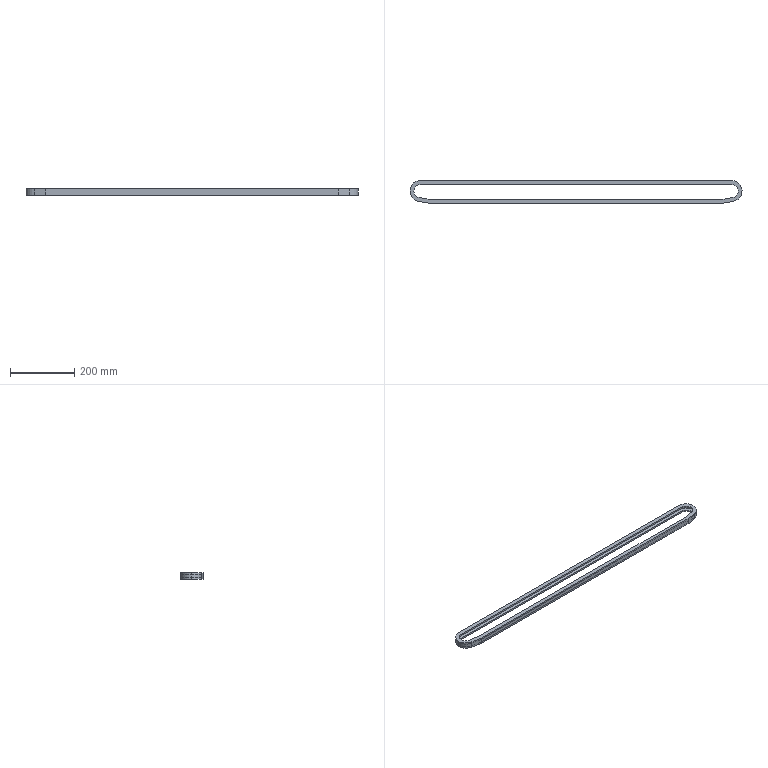Part | SolidWorks | features Extrusion 1, ICE 1 | 1 solid | 32 faces | box 1035 x 70.699 x 20 mm | volume 274324 mm3 | plane 20 | cylinder 12 | commonest cylinder face diameters 41 x6 63 x3 65 x3
STEP:
#1=CARTESIAN_POINT('',(516.5,0.,-5.));
#2=VERTEX_POINT('',#1);
#3=CARTESIAN_POINT('',(485.,31.5,-5.));
#4=VERTEX_POINT('',#3);
#5=CARTESIAN_POINT('',(485.,0.,-5.));
#6=DIRECTION('',(0.,0.,1.));
#7=DIRECTION('',(1.,0.,0.));
#8=AXIS2_PLACEMENT_3D('',#5,#6,#7);
#9=CIRCLE('',#8,31.5);
#10=EDGE_CURVE('',#2,#4,#9,.T.);
#11=ORIENTED_EDGE('',*,*,#10,.F.);
#12=CARTESIAN_POINT('',(516.5,0.,5.));
#13=VERTEX_POINT('',#12);
#14=CARTESIAN_POINT('',(516.5,0.,-5.));
#15=DIRECTION('',(0.,0.,1.));
#16=VECTOR('',#15,1000.);
#17=LINE('',#14,#16);
#18=EDGE_CURVE('',#2,#13,#17,.T.);
#19=ORIENTED_EDGE('',*,*,#18,.T.);
#20=CARTESIAN_POINT('',(485.,31.5,5.));
#21=VERTEX_POINT('',#20);
#22=CARTESIAN_POINT('',(485.,0.,5.));
#23=DIRECTION('',(0.,0.,1.));
#24=DIRECTION('',(1.,0.,0.));
#25=AXIS2_PLACEMENT_3D('',#22,#23,#24);
#26=CIRCLE('',#25,31.5);
#27=EDGE_CURVE('',#13,#21,#26,.T.);
#28=ORIENTED_EDGE('',*,*,#27,.T.);
#29=CARTESIAN_POINT('',(485.,31.5,-5.));
#30=DIRECTION('',(0.,0.,1.));
#31=VECTOR('',#30,1000.);
#32=LINE('',#29,#31);
#33=EDGE_CURVE('',#4,#21,#32,.T.);
#34=ORIENTED_EDGE('',*,*,#33,.F.);
#35=EDGE_LOOP('',(#11,#19,#28,#34));
#36=FACE_OUTER_BOUND('',#35,.T.);
#37=CARTESIAN_POINT('',(485.,0.,-5.));
#38=DIRECTION('',(0.,0.,1.));
#39=DIRECTION('',(1.,0.,0.));
#40=AXIS2_PLACEMENT_3D('',#37,#38,#39);
#41=CYLINDRICAL_SURFACE('',#40,31.5);
#42=ADVANCED_FACE('',(#36),#41,.F.);
#43=CARTESIAN_POINT('',(-485.,20.5,10.));
#44=VERTEX_POINT('',#43);
#45=CARTESIAN_POINT('',(-505.5,0.,10.));
#46=VERTEX_POINT('',#45);
#47=CARTESIAN_POINT('',(-485.,0.,10.));
#48=DIRECTION('',(0.,0.,1.));
#49=DIRECTION('',(1.,0.,0.));
#50=AXIS2_PLACEMENT_3D('',#47,#48,#49);
#51=CIRCLE('',#50,20.5);
#52=EDGE_CURVE('',#44,#46,#51,.T.);
#53=ORIENTED_EDGE('',*,*,#52,.T.);
#54=CARTESIAN_POINT('',(-505.5,0.,5.));
#55=VERTEX_POINT('',#54);
#56=CARTESIAN_POINT('',(-505.5,0.,10.));
#57=DIRECTION('',(0.,0.,-1.));
#58=VECTOR('',#57,1000.);
#59=LINE('',#56,#58);
#60=EDGE_CURVE('',#46,#55,#59,.T.);
#61=ORIENTED_EDGE('',*,*,#60,.T.);
#62=CARTESIAN_POINT('',(-485.,20.5,5.));
#63=VERTEX_POINT('',#62);
#64=CARTESIAN_POINT('',(-485.,0.,5.));
#65=DIRECTION('',(0.,0.,1.));
#66=DIRECTION('',(1.,0.,0.));
#67=AXIS2_PLACEMENT_3D('',#64,#65,#66);
#68=CIRCLE('',#67,20.5);
#69=EDGE_CURVE('',#63,#55,#68,.T.);
#70=ORIENTED_EDGE('',*,*,#69,.F.);
#71=CARTESIAN_POINT('',(-485.,20.5,10.));
#72=DIRECTION('',(0.,0.,-1.));
#73=VECTOR('',#72,1000.);
#74=LINE('',#71,#73);
#75=EDGE_CURVE('',#44,#63,#74,.T.);
#76=ORIENTED_EDGE('',*,*,#75,.F.);
#77=EDGE_LOOP('',(#53,#61,#70,#76));
#78=FACE_OUTER_BOUND('',#77,.T.);
#79=CARTESIAN_POINT('',(-485.,0.,10.));
#80=DIRECTION('',(0.,0.,-1.));
#81=DIRECTION('',(-1.,0.,0.));
#82=AXIS2_PLACEMENT_3D('',#79,#80,#81);
#83=CYLINDRICAL_SURFACE('',#82,20.5);
#84=ADVANCED_FACE('',(#78),#83,.F.);
#85=CARTESIAN_POINT('',(-517.5,0.,10.));
#86=VERTEX_POINT('',#85);
#87=CARTESIAN_POINT('',(-490.644,-32.006,10.));
#88=VERTEX_POINT('',#87);
#89=CARTESIAN_POINT('',(-485.,0.,10.));
#90=DIRECTION('',(0.,0.,1.));
#91=DIRECTION('',(1.,0.,0.));
#92=AXIS2_PLACEMENT_3D('',#89,#90,#91);
#93=CIRCLE('',#92,32.5);
#94=EDGE_CURVE('',#86,#88,#93,.T.);
#95=ORIENTED_EDGE('',*,*,#94,.F.);
#96=CARTESIAN_POINT('',(-517.5,0.,-10.));
#97=VERTEX_POINT('',#96);
#98=CARTESIAN_POINT('',(-517.5,0.,10.));
#99=DIRECTION('',(0.,0.,-1.));
#100=VECTOR('',#99,1000.);
#101=LINE('',#98,#100);
#102=EDGE_CURVE('',#86,#97,#101,.T.);
#103=ORIENTED_EDGE('',*,*,#102,.T.);
#104=CARTESIAN_POINT('',(-490.644,-32.006,-10.));
#105=VERTEX_POINT('',#104);
#106=CARTESIAN_POINT('',(-485.,0.,-10.));
#107=DIRECTION('',(0.,0.,1.));
#108=DIRECTION('',(1.,0.,0.));
#109=AXIS2_PLACEMENT_3D('',#106,#107,#108);
#110=CIRCLE('',#109,32.5);
#111=EDGE_CURVE('',#97,#105,#110,.T.);
#112=ORIENTED_EDGE('',*,*,#111,.T.);
#113=CARTESIAN_POINT('',(-490.644,-32.006,10.));
#114=DIRECTION('',(0.,0.,-1.));
#115=VECTOR('',#114,1000.);
#116=LINE('',#113,#115);
#117=EDGE_CURVE('',#88,#105,#116,.T.);
#118=ORIENTED_EDGE('',*,*,#117,.F.);
#119=EDGE_LOOP('',(#95,#103,#112,#118));
#120=FACE_OUTER_BOUND('',#119,.T.);
#121=CARTESIAN_POINT('',(-485.,0.,10.));
#122=DIRECTION('',(0.,0.,-1.));
#123=DIRECTION('',(-1.,0.,0.));
#124=AXIS2_PLACEMENT_3D('',#121,#122,#123);
#125=CYLINDRICAL_SURFACE('',#124,32.5);
#126=ADVANCED_FACE('',(#120),#125,.T.);
#127=CARTESIAN_POINT('',(-485.,20.5,-5.));
#128=VERTEX_POINT('',#127);
#129=CARTESIAN_POINT('',(-505.5,0.,-5.));
#130=VERTEX_POINT('',#129);
#131=CARTESIAN_POINT('',(-485.,0.,-5.));
#132=DIRECTION('',(0.,0.,1.));
#133=DIRECTION('',(1.,0.,0.));
#134=AXIS2_PLACEMENT_3D('',#131,#132,#133);
#135=CIRCLE('',#134,20.5);
#136=EDGE_CURVE('',#128,#130,#135,.T.);
#137=ORIENTED_EDGE('',*,*,#136,.T.);
#138=CARTESIAN_POINT('',(-505.5,0.,-10.));
#139=VERTEX_POINT('',#138);
#140=CARTESIAN_POINT('',(-505.5,0.,10.));
#141=DIRECTION('',(0.,0.,-1.));
#142=VECTOR('',#141,1000.);
#143=LINE('',#140,#142);
#144=EDGE_CURVE('',#130,#139,#143,.T.);
#145=ORIENTED_EDGE('',*,*,#144,.T.);
#146=CARTESIAN_POINT('',(-485.,20.5,-10.));
#147=VERTEX_POINT('',#146);
#148=CARTESIAN_POINT('',(-485.,0.,-10.));
#149=DIRECTION('',(0.,0.,1.));
#150=DIRECTION('',(1.,0.,0.));
#151=AXIS2_PLACEMENT_3D('',#148,#149,#150);
#152=CIRCLE('',#151,20.5);
#153=EDGE_CURVE('',#147,#139,#152,.T.);
#154=ORIENTED_EDGE('',*,*,#153,.F.);
#155=CARTESIAN_POINT('',(-485.,20.5,10.));
#156=DIRECTION('',(0.,0.,-1.));
#157=VECTOR('',#156,1000.);
#158=LINE('',#155,#157);
#159=EDGE_CURVE('',#128,#147,#158,.T.);
#160=ORIENTED_EDGE('',*,*,#159,.F.);
#161=EDGE_LOOP('',(#137,#145,#154,#160));
#162=FACE_OUTER_BOUND('',#161,.T.);
#163=CARTESIAN_POINT('',(-485.,0.,10.));
#164=DIRECTION('',(0.,0.,-1.));
#165=DIRECTION('',(-1.,0.,0.));
#166=AXIS2_PLACEMENT_3D('',#163,#164,#165);
#167=CYLINDRICAL_SURFACE('',#166,20.5);
#168=ADVANCED_FACE('',(#162),#167,.F.);
#169=ORIENTED_EDGE('',*,*,#144,.F.);
#170=CARTESIAN_POINT('',(-488.56,-20.189,-5.));
#171=VERTEX_POINT('',#170);
#172=CARTESIAN_POINT('',(-485.,0.,-5.));
#173=DIRECTION('',(0.,0.,1.));
#174=DIRECTION('',(1.,0.,0.));
#175=AXIS2_PLACEMENT_3D('',#172,#173,#174);
#176=CIRCLE('',#175,20.5);
#177=EDGE_CURVE('',#130,#171,#176,.T.);
#178=ORIENTED_EDGE('',*,*,#177,.T.);
#179=CARTESIAN_POINT('',(-488.56,-20.189,-10.));
#180=VERTEX_POINT('',#179);
#181=CARTESIAN_POINT('',(-488.56,-20.189,10.));
#182=DIRECTION('',(0.,0.,-1.));
#183=VECTOR('',#182,1000.);
#184=LINE('',#181,#183);
#185=EDGE_CURVE('',#171,#180,#184,.T.);
#186=ORIENTED_EDGE('',*,*,#185,.T.);
#187=CARTESIAN_POINT('',(-485.,0.,-10.));
#188=DIRECTION('',(0.,0.,1.));
#189=DIRECTION('',(1.,0.,0.));
#190=AXIS2_PLACEMENT_3D('',#187,#188,#189);
#191=CIRCLE('',#190,20.5);
#192=EDGE_CURVE('',#139,#180,#191,.T.);
#193=ORIENTED_EDGE('',*,*,#192,.F.);
#194=EDGE_LOOP('',(#169,#178,#186,#193));
#195=FACE_OUTER_BOUND('',#194,.T.);
#196=CARTESIAN_POINT('',(-485.,0.,10.));
#197=DIRECTION('',(0.,0.,-1.));
#198=DIRECTION('',(-1.,0.,0.));
#199=AXIS2_PLACEMENT_3D('',#196,#197,#198);
#200=CYLINDRICAL_SURFACE('',#199,20.5);
#201=ADVANCED_FACE('',(#195),#200,.F.);
#202=ORIENTED_EDGE('',*,*,#185,.F.);
#203=CARTESIAN_POINT('',(-454.475,-26.199,-5.));
#204=VERTEX_POINT('',#203);
#205=CARTESIAN_POINT('',(-454.475,-26.199,-5.));
#206=DIRECTION('',(0.9848,-0.1736,0.));
#207=VECTOR('',#206,1000.);
#208=LINE('',#205,#207);
#209=EDGE_CURVE('',#171,#204,#208,.T.);
#210=ORIENTED_EDGE('',*,*,#209,.T.);
#211=CARTESIAN_POINT('',(-454.475,-26.199,-10.));
#212=VERTEX_POINT('',#211);
#213=CARTESIAN_POINT('',(-454.475,-26.199,10.));
#214=DIRECTION('',(0.,0.,-1.));
#215=VECTOR('',#214,1000.);
#216=LINE('',#213,#215);
#217=EDGE_CURVE('',#204,#212,#216,.T.);
#218=ORIENTED_EDGE('',*,*,#217,.T.);
#219=CARTESIAN_POINT('',(-454.475,-26.199,-10.));
#220=DIRECTION('',(0.9848,-0.1736,0.));
#221=VECTOR('',#220,1000.);
#222=LINE('',#219,#221);
#223=EDGE_CURVE('',#180,#212,#222,.T.);
#224=ORIENTED_EDGE('',*,*,#223,.F.);
#225=EDGE_LOOP('',(#202,#210,#218,#224));
#226=FACE_OUTER_BOUND('',#225,.T.);
#227=CARTESIAN_POINT('',(-454.475,-26.199,10.));
#228=DIRECTION('',(0.1736,0.9848,0.));
#229=DIRECTION('',(-0.9848,0.1736,0.));
#230=AXIS2_PLACEMENT_3D('',#227,#228,#229);
#231=PLANE('',#230);
#232=ADVANCED_FACE('',(#226),#231,.T.);
#233=ORIENTED_EDGE('',*,*,#217,.F.);
#234=CARTESIAN_POINT('',(454.475,-26.199,-5.));
#235=VERTEX_POINT('',#234);
#236=CARTESIAN_POINT('',(-454.475,-26.199,-5.));
#237=DIRECTION('',(1.,0.,0.));
#238=VECTOR('',#237,1000.);
#239=LINE('',#236,#238);
#240=EDGE_CURVE('',#204,#235,#239,.T.);
#241=ORIENTED_EDGE('',*,*,#240,.T.);
#242=CARTESIAN_POINT('',(454.475,-26.199,-10.));
#243=VERTEX_POINT('',#242);
#244=CARTESIAN_POINT('',(454.475,-26.199,10.));
#245=DIRECTION('',(0.,0.,-1.));
#246=VECTOR('',#245,1000.);
#247=LINE('',#244,#246);
#248=EDGE_CURVE('',#235,#243,#247,.T.);
#249=ORIENTED_EDGE('',*,*,#248,.T.);
#250=CARTESIAN_POINT('',(-454.475,-26.199,-10.));
#251=DIRECTION('',(1.,0.,0.));
#252=VECTOR('',#251,1000.);
#253=LINE('',#250,#252);
#254=EDGE_CURVE('',#212,#243,#253,.T.);
#255=ORIENTED_EDGE('',*,*,#254,.F.);
#256=EDGE_LOOP('',(#233,#241,#249,#255));
#257=FACE_OUTER_BOUND('',#256,.T.);
#258=CARTESIAN_POINT('',(-454.475,-26.199,10.));
#259=DIRECTION('',(0.,1.,0.));
#260=DIRECTION('',(0.,0.,1.));
#261=AXIS2_PLACEMENT_3D('',#258,#259,#260);
#262=PLANE('',#261);
#263=ADVANCED_FACE('',(#257),#262,.T.);
#264=ORIENTED_EDGE('',*,*,#248,.F.);
#265=CARTESIAN_POINT('',(488.56,-20.189,-5.));
#266=VERTEX_POINT('',#265);
#267=CARTESIAN_POINT('',(454.475,-26.199,-5.));
#268=DIRECTION('',(0.9848,0.1736,0.));
#269=VECTOR('',#268,1000.);
#270=LINE('',#267,#269);
#271=EDGE_CURVE('',#235,#266,#270,.T.);
#272=ORIENTED_EDGE('',*,*,#271,.T.);
#273=CARTESIAN_POINT('',(488.56,-20.189,-10.));
#274=VERTEX_POINT('',#273);
#275=CARTESIAN_POINT('',(488.56,-20.189,10.));
#276=DIRECTION('',(0.,0.,-1.));
#277=VECTOR('',#276,1000.);
#278=LINE('',#275,#277);
#279=EDGE_CURVE('',#266,#274,#278,.T.);
#280=ORIENTED_EDGE('',*,*,#279,.T.);
#281=CARTESIAN_POINT('',(454.475,-26.199,-10.));
#282=DIRECTION('',(0.9848,0.1736,0.));
#283=VECTOR('',#282,1000.);
#284=LINE('',#281,#283);
#285=EDGE_CURVE('',#243,#274,#284,.T.);
#286=ORIENTED_EDGE('',*,*,#285,.F.);
#287=EDGE_LOOP('',(#264,#272,#280,#286));
#288=FACE_OUTER_BOUND('',#287,.T.);
#289=CARTESIAN_POINT('',(454.475,-26.199,10.));
#290=DIRECTION('',(-0.1736,0.9848,0.));
#291=DIRECTION('',(-0.9848,-0.1736,0.));
#292=AXIS2_PLACEMENT_3D('',#289,#290,#291);
#293=PLANE('',#292);
#294=ADVANCED_FACE('',(#288),#293,.T.);
#295=ORIENTED_EDGE('',*,*,#279,.F.);
#296=CARTESIAN_POINT('',(485.,20.5,-5.));
#297=VERTEX_POINT('',#296);
#298=CARTESIAN_POINT('',(485.,0.,-5.));
#299=DIRECTION('',(0.,0.,1.));
#300=DIRECTION('',(1.,0.,0.));
#301=AXIS2_PLACEMENT_3D('',#298,#299,#300);
#302=CIRCLE('',#301,20.5);
#303=EDGE_CURVE('',#266,#297,#302,.T.);
#304=ORIENTED_EDGE('',*,*,#303,.T.);
#305=CARTESIAN_POINT('',(485.,20.5,-10.));
#306=VERTEX_POINT('',#305);
#307=CARTESIAN_POINT('',(485.,20.5,10.));
#308=DIRECTION('',(0.,0.,-1.));
#309=VECTOR('',#308,1000.);
#310=LINE('',#307,#309);
#311=EDGE_CURVE('',#297,#306,#310,.T.);
#312=ORIENTED_EDGE('',*,*,#311,.T.);
#313=CARTESIAN_POINT('',(485.,0.,-10.));
#314=DIRECTION('',(0.,0.,1.));
#315=DIRECTION('',(-1.,0.,0.));
#316=AXIS2_PLACEMENT_3D('',#313,#314,#315);
#317=CIRCLE('',#316,20.5);
#318=EDGE_CURVE('',#274,#306,#317,.T.);
#319=ORIENTED_EDGE('',*,*,#318,.F.);
#320=EDGE_LOOP('',(#295,#304,#312,#319));
#321=FACE_OUTER_BOUND('',#320,.T.);
#322=CARTESIAN_POINT('',(485.,0.,10.));
#323=DIRECTION('',(0.,0.,-1.));
#324=DIRECTION('',(-1.,0.,0.));
#325=AXIS2_PLACEMENT_3D('',#322,#323,#324);
#326=CYLINDRICAL_SURFACE('',#325,20.5);
#327=ADVANCED_FACE('',(#321),#326,.F.);
#328=ORIENTED_EDGE('',*,*,#311,.F.);
#329=CARTESIAN_POINT('',(-485.,20.5,-5.));
#330=DIRECTION('',(-1.,0.,0.));
#331=VECTOR('',#330,1000.);
#332=LINE('',#329,#331);
#333=EDGE_CURVE('',#297,#128,#332,.T.);
#334=ORIENTED_EDGE('',*,*,#333,.T.);
#335=ORIENTED_EDGE('',*,*,#159,.T.);
#336=CARTESIAN_POINT('',(-485.,20.5,-10.));
#337=DIRECTION('',(-1.,0.,0.));
#338=VECTOR('',#337,1000.);
#339=LINE('',#336,#338);
#340=EDGE_CURVE('',#306,#147,#339,.T.);
#341=ORIENTED_EDGE('',*,*,#340,.F.);
#342=EDGE_LOOP('',(#328,#334,#335,#341));
#343=FACE_OUTER_BOUND('',#342,.T.);
#344=CARTESIAN_POINT('',(-485.,20.5,10.));
#345=DIRECTION('',(0.,-1.,0.));
#346=DIRECTION('',(0.,0.,-1.));
#347=AXIS2_PLACEMENT_3D('',#344,#345,#346);
#348=PLANE('',#347);
#349=ADVANCED_FACE('',(#343),#348,.T.);
#350=CARTESIAN_POINT('',(-485.,32.5,10.));
#351=VERTEX_POINT('',#350);
#352=CARTESIAN_POINT('',(-485.,0.,10.));
#353=DIRECTION('',(0.,0.,1.));
#354=DIRECTION('',(1.,0.,0.));
#355=AXIS2_PLACEMENT_3D('',#352,#353,#354);
#356=CIRCLE('',#355,32.5);
#357=EDGE_CURVE('',#351,#86,#356,.T.);
#358=ORIENTED_EDGE('',*,*,#357,.T.);
#359=ORIENTED_EDGE('',*,*,#94,.T.);
#360=CARTESIAN_POINT('',(-455.525,-38.199,10.));
#361=VERTEX_POINT('',#360);
#362=CARTESIAN_POINT('',(-455.525,-38.199,10.));
#363=DIRECTION('',(0.9848,-0.1736,0.));
#364=VECTOR('',#363,1000.);
#365=LINE('',#362,#364);
#366=EDGE_CURVE('',#88,#361,#365,.T.);
#367=ORIENTED_EDGE('',*,*,#366,.T.);
#368=CARTESIAN_POINT('',(455.525,-38.199,10.));
#369=VERTEX_POINT('',#368);
#370=CARTESIAN_POINT('',(-455.525,-38.199,10.));
#371=DIRECTION('',(1.,0.,0.));
#372=VECTOR('',#371,1000.);
#373=LINE('',#370,#372);
#374=EDGE_CURVE('',#361,#369,#373,.T.);
#375=ORIENTED_EDGE('',*,*,#374,.T.);
#376=CARTESIAN_POINT('',(490.644,-32.006,10.));
#377=VERTEX_POINT('',#376);
#378=CARTESIAN_POINT('',(455.525,-38.199,10.));
#379=DIRECTION('',(0.9848,0.1736,0.));
#380=VECTOR('',#379,1000.);
#381=LINE('',#378,#380);
#382=EDGE_CURVE('',#369,#377,#381,.T.);
#383=ORIENTED_EDGE('',*,*,#382,.T.);
#384=CARTESIAN_POINT('',(485.,32.5,10.));
#385=VERTEX_POINT('',#384);
#386=CARTESIAN_POINT('',(485.,0.,10.));
#387=DIRECTION('',(0.,0.,1.));
#388=DIRECTION('',(-1.,0.,0.));
#389=AXIS2_PLACEMENT_3D('',#386,#387,#388);
#390=CIRCLE('',#389,32.5);
#391=EDGE_CURVE('',#377,#385,#390,.T.);
#392=ORIENTED_EDGE('',*,*,#391,.T.);
#393=CARTESIAN_POINT('',(-485.,32.5,10.));
#394=DIRECTION('',(-1.,0.,0.));
#395=VECTOR('',#394,1000.);
#396=LINE('',#393,#395);
#397=EDGE_CURVE('',#385,#351,#396,.T.);
#398=ORIENTED_EDGE('',*,*,#397,.T.);
#399=EDGE_LOOP('',(#358,#359,#367,#375,#383,#392,#398));
#400=FACE_OUTER_BOUND('',#399,.T.);
#401=CARTESIAN_POINT('',(-488.56,-20.189,10.));
#402=VERTEX_POINT('',#401);
#403=CARTESIAN_POINT('',(-454.475,-26.199,10.));
#404=VERTEX_POINT('',#403);
#405=CARTESIAN_POINT('',(-454.475,-26.199,10.));
#406=DIRECTION('',(0.9848,-0.1736,0.));
#407=VECTOR('',#406,1000.);
#408=LINE('',#405,#407);
#409=EDGE_CURVE('',#402,#404,#408,.T.);
#410=ORIENTED_EDGE('',*,*,#409,.F.);
#411=CARTESIAN_POINT('',(-485.,0.,10.));
#412=DIRECTION('',(0.,0.,1.));
#413=DIRECTION('',(1.,0.,0.));
#414=AXIS2_PLACEMENT_3D('',#411,#412,#413);
#415=CIRCLE('',#414,20.5);
#416=EDGE_CURVE('',#46,#402,#415,.T.);
#417=ORIENTED_EDGE('',*,*,#416,.F.);
#418=ORIENTED_EDGE('',*,*,#52,.F.);
#419=CARTESIAN_POINT('',(485.,20.5,10.));
#420=VERTEX_POINT('',#419);
#421=CARTESIAN_POINT('',(-485.,20.5,10.));
#422=DIRECTION('',(-1.,0.,0.));
#423=VECTOR('',#422,1000.);
#424=LINE('',#421,#423);
#425=EDGE_CURVE('',#420,#44,#424,.T.);
#426=ORIENTED_EDGE('',*,*,#425,.F.);
#427=CARTESIAN_POINT('',(488.56,-20.189,10.));
#428=VERTEX_POINT('',#427);
#429=CARTESIAN_POINT('',(485.,0.,10.));
#430=DIRECTION('',(0.,0.,1.));
#431=DIRECTION('',(-1.,0.,0.));
#432=AXIS2_PLACEMENT_3D('',#429,#430,#431);
#433=CIRCLE('',#432,20.5);
#434=EDGE_CURVE('',#428,#420,#433,.T.);
#435=ORIENTED_EDGE('',*,*,#434,.F.);
#436=CARTESIAN_POINT('',(454.475,-26.199,10.));
#437=VERTEX_POINT('',#436);
#438=CARTESIAN_POINT('',(454.475,-26.199,10.));
#439=DIRECTION('',(0.9848,0.1736,0.));
#440=VECTOR('',#439,1000.);
#441=LINE('',#438,#440);
#442=EDGE_CURVE('',#437,#428,#441,.T.);
#443=ORIENTED_EDGE('',*,*,#442,.F.);
#444=CARTESIAN_POINT('',(-454.475,-26.199,10.));
#445=DIRECTION('',(1.,0.,0.));
#446=VECTOR('',#445,1000.);
#447=LINE('',#444,#446);
#448=EDGE_CURVE('',#404,#437,#447,.T.);
#449=ORIENTED_EDGE('',*,*,#448,.F.);
#450=EDGE_LOOP('',(#410,#417,#418,#426,#435,#443,#449));
#451=FACE_BOUND('',#450,.T.);
#452=CARTESIAN_POINT('',(-485.,0.,10.));
#453=DIRECTION('',(0.,0.,1.));
#454=DIRECTION('',(1.,0.,0.));
#455=AXIS2_PLACEMENT_3D('',#452,#453,#454);
#456=PLANE('',#455);
#457=ADVANCED_FACE('',(#400,#451),#456,.T.);
#458=CARTESIAN_POINT('',(-485.,32.5,-10.));
#459=VERTEX_POINT('',#458);
#460=CARTESIAN_POINT('',(-485.,0.,-10.));
#461=DIRECTION('',(0.,0.,1.));
#462=DIRECTION('',(1.,0.,0.));
#463=AXIS2_PLACEMENT_3D('',#460,#461,#462);
#464=CIRCLE('',#463,32.5);
#465=EDGE_CURVE('',#459,#97,#464,.T.);
#466=ORIENTED_EDGE('',*,*,#465,.F.);
#467=CARTESIAN_POINT('',(485.,32.5,-10.));
#468=VERTEX_POINT('',#467);
#469=CARTESIAN_POINT('',(-485.,32.5,-10.));
#470=DIRECTION('',(-1.,0.,0.));
#471=VECTOR('',#470,1000.);
#472=LINE('',#469,#471);
#473=EDGE_CURVE('',#468,#459,#472,.T.);
#474=ORIENTED_EDGE('',*,*,#473,.F.);
#475=CARTESIAN_POINT('',(490.644,-32.006,-10.));
#476=VERTEX_POINT('',#475);
#477=CARTESIAN_POINT('',(485.,0.,-10.));
#478=DIRECTION('',(0.,0.,1.));
#479=DIRECTION('',(-1.,0.,0.));
#480=AXIS2_PLACEMENT_3D('',#477,#478,#479);
#481=CIRCLE('',#480,32.5);
#482=EDGE_CURVE('',#476,#468,#481,.T.);
#483=ORIENTED_EDGE('',*,*,#482,.F.);
#484=CARTESIAN_POINT('',(455.525,-38.199,-10.));
#485=VERTEX_POINT('',#484);
#486=CARTESIAN_POINT('',(455.525,-38.199,-10.));
#487=DIRECTION('',(0.9848,0.1736,0.));
#488=VECTOR('',#487,1000.);
#489=LINE('',#486,#488);
#490=EDGE_CURVE('',#485,#476,#489,.T.);
#491=ORIENTED_EDGE('',*,*,#490,.F.);
#492=CARTESIAN_POINT('',(-455.525,-38.199,-10.));
#493=VERTEX_POINT('',#492);
#494=CARTESIAN_POINT('',(-455.525,-38.199,-10.));
#495=DIRECTION('',(1.,0.,0.));
#496=VECTOR('',#495,1000.);
#497=LINE('',#494,#496);
#498=EDGE_CURVE('',#493,#485,#497,.T.);
#499=ORIENTED_EDGE('',*,*,#498,.F.);
#500=CARTESIAN_POINT('',(-455.525,-38.199,-10.));
#501=DIRECTION('',(0.9848,-0.1736,0.));
#502=VECTOR('',#501,1000.);
#503=LINE('',#500,#502);
#504=EDGE_CURVE('',#105,#493,#503,.T.);
#505=ORIENTED_EDGE('',*,*,#504,.F.);
#506=ORIENTED_EDGE('',*,*,#111,.F.);
#507=EDGE_LOOP('',(#466,#474,#483,#491,#499,#505,#506));
#508=FACE_OUTER_BOUND('',#507,.T.);
#509=ORIENTED_EDGE('',*,*,#153,.T.);
#510=ORIENTED_EDGE('',*,*,#192,.T.);
#511=ORIENTED_EDGE('',*,*,#223,.T.);
#512=ORIENTED_EDGE('',*,*,#254,.T.);
#513=ORIENTED_EDGE('',*,*,#285,.T.);
#514=ORIENTED_EDGE('',*,*,#318,.T.);
#515=ORIENTED_EDGE('',*,*,#340,.T.);
#516=EDGE_LOOP('',(#509,#510,#511,#512,#513,#514,#515));
#517=FACE_BOUND('',#516,.T.);
#518=CARTESIAN_POINT('',(-485.,0.,-10.));
#519=DIRECTION('',(0.,0.,1.));
#520=DIRECTION('',(1.,0.,0.));
#521=AXIS2_PLACEMENT_3D('',#518,#519,#520);
#522=PLANE('',#521);
#523=ADVANCED_FACE('',(#508,#517),#522,.F.);
#524=ORIENTED_EDGE('',*,*,#102,.F.);
#525=ORIENTED_EDGE('',*,*,#357,.F.);
#526=CARTESIAN_POINT('',(-485.,32.5,10.));
#527=DIRECTION('',(0.,0.,-1.));
#528=VECTOR('',#527,1000.);
#529=LINE('',#526,#528);
#530=EDGE_CURVE('',#351,#459,#529,.T.);
#531=ORIENTED_EDGE('',*,*,#530,.T.);
#532=ORIENTED_EDGE('',*,*,#465,.T.);
#533=EDGE_LOOP('',(#524,#525,#531,#532));
#534=FACE_OUTER_BOUND('',#533,.T.);
#535=CARTESIAN_POINT('',(-485.,0.,10.));
#536=DIRECTION('',(0.,0.,-1.));
#537=DIRECTION('',(-1.,0.,0.));
#538=AXIS2_PLACEMENT_3D('',#535,#536,#537);
#539=CYLINDRICAL_SURFACE('',#538,32.5);
#540=ADVANCED_FACE('',(#534),#539,.T.);
#541=ORIENTED_EDGE('',*,*,#504,.T.);
#542=CARTESIAN_POINT('',(-455.525,-38.199,10.));
#543=DIRECTION('',(0.,0.,-1.));
#544=VECTOR('',#543,1000.);
#545=LINE('',#542,#544);
#546=EDGE_CURVE('',#361,#493,#545,.T.);
#547=ORIENTED_EDGE('',*,*,#546,.F.);
#548=ORIENTED_EDGE('',*,*,#366,.F.);
#549=ORIENTED_EDGE('',*,*,#117,.T.);
#550=EDGE_LOOP('',(#541,#547,#548,#549));
#551=FACE_OUTER_BOUND('',#550,.T.);
#552=CARTESIAN_POINT('',(-455.525,-38.199,10.));
#553=DIRECTION('',(0.1736,0.9848,0.));
#554=DIRECTION('',(-0.9848,0.1736,0.));
#555=AXIS2_PLACEMENT_3D('',#552,#553,#554);
#556=PLANE('',#555);
#557=ADVANCED_FACE('',(#551),#556,.F.);
#558=ORIENTED_EDGE('',*,*,#498,.T.);
#559=CARTESIAN_POINT('',(455.525,-38.199,10.));
#560=DIRECTION('',(0.,0.,-1.));
#561=VECTOR('',#560,1000.);
#562=LINE('',#559,#561);
#563=EDGE_CURVE('',#369,#485,#562,.T.);
#564=ORIENTED_EDGE('',*,*,#563,.F.);
#565=ORIENTED_EDGE('',*,*,#374,.F.);
#566=ORIENTED_EDGE('',*,*,#546,.T.);
#567=EDGE_LOOP('',(#558,#564,#565,#566));
#568=FACE_OUTER_BOUND('',#567,.T.);
#569=CARTESIAN_POINT('',(-455.525,-38.199,10.));
#570=DIRECTION('',(0.,1.,0.));
#571=DIRECTION('',(0.,0.,1.));
#572=AXIS2_PLACEMENT_3D('',#569,#570,#571);
#573=PLANE('',#572);
#574=ADVANCED_FACE('',(#568),#573,.F.);
#575=ORIENTED_EDGE('',*,*,#490,.T.);
#576=CARTESIAN_POINT('',(490.644,-32.006,10.));
#577=DIRECTION('',(0.,0.,-1.));
#578=VECTOR('',#577,1000.);
#579=LINE('',#576,#578);
#580=EDGE_CURVE('',#377,#476,#579,.T.);
#581=ORIENTED_EDGE('',*,*,#580,.F.);
#582=ORIENTED_EDGE('',*,*,#382,.F.);
#583=ORIENTED_EDGE('',*,*,#563,.T.);
#584=EDGE_LOOP('',(#575,#581,#582,#583));
#585=FACE_OUTER_BOUND('',#584,.T.);
#586=CARTESIAN_POINT('',(455.525,-38.199,10.));
#587=DIRECTION('',(-0.1736,0.9848,0.));
#588=DIRECTION('',(-0.9848,-0.1736,0.));
#589=AXIS2_PLACEMENT_3D('',#586,#587,#588);
#590=PLANE('',#589);
#591=ADVANCED_FACE('',(#585),#590,.F.);
#592=ORIENTED_EDGE('',*,*,#482,.T.);
#593=CARTESIAN_POINT('',(485.,32.5,10.));
#594=DIRECTION('',(0.,0.,-1.));
#595=VECTOR('',#594,1000.);
#596=LINE('',#593,#595);
#597=EDGE_CURVE('',#385,#468,#596,.T.);
#598=ORIENTED_EDGE('',*,*,#597,.F.);
#599=ORIENTED_EDGE('',*,*,#391,.F.);
#600=ORIENTED_EDGE('',*,*,#580,.T.);
#601=EDGE_LOOP('',(#592,#598,#599,#600));
#602=FACE_OUTER_BOUND('',#601,.T.);
#603=CARTESIAN_POINT('',(485.,0.,10.));
#604=DIRECTION('',(0.,0.,-1.));
#605=DIRECTION('',(-1.,0.,0.));
#606=AXIS2_PLACEMENT_3D('',#603,#604,#605);
#607=CYLINDRICAL_SURFACE('',#606,32.5);
#608=ADVANCED_FACE('',(#602),#607,.T.);
#609=ORIENTED_EDGE('',*,*,#473,.T.);
#610=ORIENTED_EDGE('',*,*,#530,.F.);
#611=ORIENTED_EDGE('',*,*,#397,.F.);
#612=ORIENTED_EDGE('',*,*,#597,.T.);
#613=EDGE_LOOP('',(#609,#610,#611,#612));
#614=FACE_OUTER_BOUND('',#613,.T.);
#615=CARTESIAN_POINT('',(-485.,32.5,10.));
#616=DIRECTION('',(0.,-1.,0.));
#617=DIRECTION('',(0.,0.,-1.));
#618=AXIS2_PLACEMENT_3D('',#615,#616,#617);
#619=PLANE('',#618);
#620=ADVANCED_FACE('',(#614),#619,.F.);
#621=ORIENTED_EDGE('',*,*,#60,.F.);
#622=ORIENTED_EDGE('',*,*,#416,.T.);
#623=CARTESIAN_POINT('',(-488.56,-20.189,5.));
#624=VERTEX_POINT('',#623);
#625=CARTESIAN_POINT('',(-488.56,-20.189,10.));
#626=DIRECTION('',(0.,0.,-1.));
#627=VECTOR('',#626,1000.);
#628=LINE('',#625,#627);
#629=EDGE_CURVE('',#402,#624,#628,.T.);
#630=ORIENTED_EDGE('',*,*,#629,.T.);
#631=CARTESIAN_POINT('',(-485.,0.,5.));
#632=DIRECTION('',(0.,0.,1.));
#633=DIRECTION('',(1.,0.,0.));
#634=AXIS2_PLACEMENT_3D('',#631,#632,#633);
#635=CIRCLE('',#634,20.5);
#636=EDGE_CURVE('',#55,#624,#635,.T.);
#637=ORIENTED_EDGE('',*,*,#636,.F.);
#638=EDGE_LOOP('',(#621,#622,#630,#637));
#639=FACE_OUTER_BOUND('',#638,.T.);
#640=CARTESIAN_POINT('',(-485.,0.,10.));
#641=DIRECTION('',(0.,0.,-1.));
#642=DIRECTION('',(-1.,0.,0.));
#643=AXIS2_PLACEMENT_3D('',#640,#641,#642);
#644=CYLINDRICAL_SURFACE('',#643,20.5);
#645=ADVANCED_FACE('',(#639),#644,.F.);
#646=CARTESIAN_POINT('',(-454.475,-26.199,5.));
#647=VERTEX_POINT('',#646);
#648=CARTESIAN_POINT('',(-454.475,-26.199,5.));
#649=DIRECTION('',(0.9848,-0.1736,0.));
#650=VECTOR('',#649,1000.);
#651=LINE('',#648,#650);
#652=EDGE_CURVE('',#624,#647,#651,.T.);
#653=ORIENTED_EDGE('',*,*,#652,.F.);
#654=ORIENTED_EDGE('',*,*,#629,.F.);
#655=ORIENTED_EDGE('',*,*,#409,.T.);
#656=CARTESIAN_POINT('',(-454.475,-26.199,10.));
#657=DIRECTION('',(0.,0.,-1.));
#658=VECTOR('',#657,1000.);
#659=LINE('',#656,#658);
#660=EDGE_CURVE('',#404,#647,#659,.T.);
#661=ORIENTED_EDGE('',*,*,#660,.T.);
#662=EDGE_LOOP('',(#653,#654,#655,#661));
#663=FACE_OUTER_BOUND('',#662,.T.);
#664=CARTESIAN_POINT('',(-454.475,-26.199,10.));
#665=DIRECTION('',(0.1736,0.9848,0.));
#666=DIRECTION('',(-0.9848,0.1736,0.));
#667=AXIS2_PLACEMENT_3D('',#664,#665,#666);
#668=PLANE('',#667);
#669=ADVANCED_FACE('',(#663),#668,.T.);
#670=CARTESIAN_POINT('',(454.475,-26.199,5.));
#671=VERTEX_POINT('',#670);
#672=CARTESIAN_POINT('',(-454.475,-26.199,5.));
#673=DIRECTION('',(1.,0.,0.));
#674=VECTOR('',#673,1000.);
#675=LINE('',#672,#674);
#676=EDGE_CURVE('',#647,#671,#675,.T.);
#677=ORIENTED_EDGE('',*,*,#676,.F.);
#678=ORIENTED_EDGE('',*,*,#660,.F.);
#679=ORIENTED_EDGE('',*,*,#448,.T.);
#680=CARTESIAN_POINT('',(454.475,-26.199,10.));
#681=DIRECTION('',(0.,0.,-1.));
#682=VECTOR('',#681,1000.);
#683=LINE('',#680,#682);
#684=EDGE_CURVE('',#437,#671,#683,.T.);
#685=ORIENTED_EDGE('',*,*,#684,.T.);
#686=EDGE_LOOP('',(#677,#678,#679,#685));
#687=FACE_OUTER_BOUND('',#686,.T.);
#688=CARTESIAN_POINT('',(-454.475,-26.199,10.));
#689=DIRECTION('',(0.,1.,0.));
#690=DIRECTION('',(0.,0.,1.));
#691=AXIS2_PLACEMENT_3D('',#688,#689,#690);
#692=PLANE('',#691);
#693=ADVANCED_FACE('',(#687),#692,.T.);
#694=CARTESIAN_POINT('',(488.56,-20.189,5.));
#695=VERTEX_POINT('',#694);
#696=CARTESIAN_POINT('',(454.475,-26.199,5.));
#697=DIRECTION('',(0.9848,0.1736,0.));
#698=VECTOR('',#697,1000.);
#699=LINE('',#696,#698);
#700=EDGE_CURVE('',#671,#695,#699,.T.);
#701=ORIENTED_EDGE('',*,*,#700,.F.);
#702=ORIENTED_EDGE('',*,*,#684,.F.);
#703=ORIENTED_EDGE('',*,*,#442,.T.);
#704=CARTESIAN_POINT('',(488.56,-20.189,10.));
#705=DIRECTION('',(0.,0.,-1.));
#706=VECTOR('',#705,1000.);
#707=LINE('',#704,#706);
#708=EDGE_CURVE('',#428,#695,#707,.T.);
#709=ORIENTED_EDGE('',*,*,#708,.T.);
#710=EDGE_LOOP('',(#701,#702,#703,#709));
#711=FACE_OUTER_BOUND('',#710,.T.);
#712=CARTESIAN_POINT('',(454.475,-26.199,10.));
#713=DIRECTION('',(-0.1736,0.9848,0.));
#714=DIRECTION('',(-0.9848,-0.1736,0.));
#715=AXIS2_PLACEMENT_3D('',#712,#713,#714);
#716=PLANE('',#715);
#717=ADVANCED_FACE('',(#711),#716,.T.);
#718=CARTESIAN_POINT('',(485.,20.5,5.));
#719=VERTEX_POINT('',#718);
#720=CARTESIAN_POINT('',(485.,0.,5.));
#721=DIRECTION('',(0.,0.,1.));
#722=DIRECTION('',(1.,0.,0.));
#723=AXIS2_PLACEMENT_3D('',#720,#721,#722);
#724=CIRCLE('',#723,20.5);
#725=EDGE_CURVE('',#695,#719,#724,.T.);
#726=ORIENTED_EDGE('',*,*,#725,.F.);
#727=ORIENTED_EDGE('',*,*,#708,.F.);
#728=ORIENTED_EDGE('',*,*,#434,.T.);
#729=CARTESIAN_POINT('',(485.,20.5,10.));
#730=DIRECTION('',(0.,0.,-1.));
#731=VECTOR('',#730,1000.);
#732=LINE('',#729,#731);
#733=EDGE_CURVE('',#420,#719,#732,.T.);
#734=ORIENTED_EDGE('',*,*,#733,.T.);
#735=EDGE_LOOP('',(#726,#727,#728,#734));
#736=FACE_OUTER_BOUND('',#735,.T.);
#737=CARTESIAN_POINT('',(485.,0.,10.));
#738=DIRECTION('',(0.,0.,-1.));
#739=DIRECTION('',(-1.,0.,0.));
#740=AXIS2_PLACEMENT_3D('',#737,#738,#739);
#741=CYLINDRICAL_SURFACE('',#740,20.5);
#742=ADVANCED_FACE('',(#736),#741,.F.);
#743=CARTESIAN_POINT('',(-485.,20.5,5.));
#744=DIRECTION('',(-1.,0.,0.));
#745=VECTOR('',#744,1000.);
#746=LINE('',#743,#745);
#747=EDGE_CURVE('',#719,#63,#746,.T.);
#748=ORIENTED_EDGE('',*,*,#747,.F.);
#749=ORIENTED_EDGE('',*,*,#733,.F.);
#750=ORIENTED_EDGE('',*,*,#425,.T.);
#751=ORIENTED_EDGE('',*,*,#75,.T.);
#752=EDGE_LOOP('',(#748,#749,#750,#751));
#753=FACE_OUTER_BOUND('',#752,.T.);
#754=CARTESIAN_POINT('',(-485.,20.5,10.));
#755=DIRECTION('',(0.,-1.,0.));
#756=DIRECTION('',(0.,0.,-1.));
#757=AXIS2_PLACEMENT_3D('',#754,#755,#756);
#758=PLANE('',#757);
#759=ADVANCED_FACE('',(#753),#758,.T.);
#760=CARTESIAN_POINT('',(-455.437,-37.199,5.));
#761=VERTEX_POINT('',#760);
#762=CARTESIAN_POINT('',(455.437,-37.199,5.));
#763=VERTEX_POINT('',#762);
#764=CARTESIAN_POINT('',(-455.437,-37.199,5.));
#765=DIRECTION('',(1.,0.,0.));
#766=VECTOR('',#765,1000.);
#767=LINE('',#764,#766);
#768=EDGE_CURVE('',#761,#763,#767,.T.);
#769=ORIENTED_EDGE('',*,*,#768,.T.);
#770=CARTESIAN_POINT('',(455.437,-37.199,-5.));
#771=VERTEX_POINT('',#770);
#772=CARTESIAN_POINT('',(455.437,-37.199,-5.));
#773=DIRECTION('',(0.,0.,1.));
#774=VECTOR('',#773,1000.);
#775=LINE('',#772,#774);
#776=EDGE_CURVE('',#771,#763,#775,.T.);
#777=ORIENTED_EDGE('',*,*,#776,.F.);
#778=CARTESIAN_POINT('',(-455.437,-37.199,-5.));
#779=VERTEX_POINT('',#778);
#780=CARTESIAN_POINT('',(-455.437,-37.199,-5.));
#781=DIRECTION('',(1.,0.,0.));
#782=VECTOR('',#781,1000.);
#783=LINE('',#780,#782);
#784=EDGE_CURVE('',#779,#771,#783,.T.);
#785=ORIENTED_EDGE('',*,*,#784,.F.);
#786=CARTESIAN_POINT('',(-455.437,-37.199,-5.));
#787=DIRECTION('',(0.,0.,1.));
#788=VECTOR('',#787,1000.);
#789=LINE('',#786,#788);
#790=EDGE_CURVE('',#779,#761,#789,.T.);
#791=ORIENTED_EDGE('',*,*,#790,.T.);
#792=EDGE_LOOP('',(#769,#777,#785,#791));
#793=FACE_OUTER_BOUND('',#792,.T.);
#794=CARTESIAN_POINT('',(-455.437,-37.199,-5.));
#795=DIRECTION('',(0.,-1.,0.));
#796=DIRECTION('',(0.,0.,-1.));
#797=AXIS2_PLACEMENT_3D('',#794,#795,#796);
#798=PLANE('',#797);
#799=ADVANCED_FACE('',(#793),#798,.F.);
#800=CARTESIAN_POINT('',(-490.47,-31.021,5.));
#801=VERTEX_POINT('',#800);
#802=CARTESIAN_POINT('',(-490.47,-31.021,5.));
#803=DIRECTION('',(0.9848,-0.1736,0.));
#804=VECTOR('',#803,1000.);
#805=LINE('',#802,#804);
#806=EDGE_CURVE('',#801,#761,#805,.T.);
#807=ORIENTED_EDGE('',*,*,#806,.T.);
#808=ORIENTED_EDGE('',*,*,#790,.F.);
#809=CARTESIAN_POINT('',(-490.47,-31.021,-5.));
#810=VERTEX_POINT('',#809);
#811=CARTESIAN_POINT('',(-490.47,-31.021,-5.));
#812=DIRECTION('',(0.9848,-0.1736,0.));
#813=VECTOR('',#812,1000.);
#814=LINE('',#811,#813);
#815=EDGE_CURVE('',#810,#779,#814,.T.);
#816=ORIENTED_EDGE('',*,*,#815,.F.);
#817=CARTESIAN_POINT('',(-490.47,-31.021,-5.));
#818=DIRECTION('',(0.,0.,1.));
#819=VECTOR('',#818,1000.);
#820=LINE('',#817,#819);
#821=EDGE_CURVE('',#810,#801,#820,.T.);
#822=ORIENTED_EDGE('',*,*,#821,.T.);
#823=EDGE_LOOP('',(#807,#808,#816,#822));
#824=FACE_OUTER_BOUND('',#823,.T.);
#825=CARTESIAN_POINT('',(-490.47,-31.021,-5.));
#826=DIRECTION('',(-0.1736,-0.9848,0.));
#827=DIRECTION('',(0.9848,-0.1736,0.));
#828=AXIS2_PLACEMENT_3D('',#825,#826,#827);
#829=PLANE('',#828);
#830=ADVANCED_FACE('',(#824),#829,.F.);
#831=CARTESIAN_POINT('',(-485.,31.5,5.));
#832=VERTEX_POINT('',#831);
#833=CARTESIAN_POINT('',(-485.,0.,5.));
#834=DIRECTION('',(0.,0.,1.));
#835=DIRECTION('',(1.,0.,0.));
#836=AXIS2_PLACEMENT_3D('',#833,#834,#835);
#837=CIRCLE('',#836,31.5);
#838=EDGE_CURVE('',#832,#801,#837,.T.);
#839=ORIENTED_EDGE('',*,*,#838,.T.);
#840=ORIENTED_EDGE('',*,*,#821,.F.);
#841=CARTESIAN_POINT('',(-485.,31.5,-5.));
#842=VERTEX_POINT('',#841);
#843=CARTESIAN_POINT('',(-485.,0.,-5.));
#844=DIRECTION('',(0.,0.,1.));
#845=DIRECTION('',(1.,0.,0.));
#846=AXIS2_PLACEMENT_3D('',#843,#844,#845);
#847=CIRCLE('',#846,31.5);
#848=EDGE_CURVE('',#842,#810,#847,.T.);
#849=ORIENTED_EDGE('',*,*,#848,.F.);
#850=CARTESIAN_POINT('',(-485.,31.5,-5.));
#851=DIRECTION('',(0.,0.,1.));
#852=VECTOR('',#851,1000.);
#853=LINE('',#850,#852);
#854=EDGE_CURVE('',#842,#832,#853,.T.);
#855=ORIENTED_EDGE('',*,*,#854,.T.);
#856=EDGE_LOOP('',(#839,#840,#849,#855));
#857=FACE_OUTER_BOUND('',#856,.T.);
#858=CARTESIAN_POINT('',(-485.,0.,-5.));
#859=DIRECTION('',(0.,0.,1.));
#860=DIRECTION('',(1.,0.,0.));
#861=AXIS2_PLACEMENT_3D('',#858,#859,#860);
#862=CYLINDRICAL_SURFACE('',#861,31.5);
#863=ADVANCED_FACE('',(#857),#862,.F.);
#864=CARTESIAN_POINT('',(485.,31.5,5.));
#865=DIRECTION('',(-1.,0.,0.));
#866=VECTOR('',#865,1000.);
#867=LINE('',#864,#866);
#868=EDGE_CURVE('',#21,#832,#867,.T.);
#869=ORIENTED_EDGE('',*,*,#868,.T.);
#870=ORIENTED_EDGE('',*,*,#854,.F.);
#871=CARTESIAN_POINT('',(485.,31.5,-5.));
#872=DIRECTION('',(-1.,0.,0.));
#873=VECTOR('',#872,1000.);
#874=LINE('',#871,#873);
#875=EDGE_CURVE('',#4,#842,#874,.T.);
#876=ORIENTED_EDGE('',*,*,#875,.F.);
#877=ORIENTED_EDGE('',*,*,#33,.T.);
#878=EDGE_LOOP('',(#869,#870,#876,#877));
#879=FACE_OUTER_BOUND('',#878,.T.);
#880=CARTESIAN_POINT('',(485.,31.5,-5.));
#881=DIRECTION('',(0.,1.,0.));
#882=DIRECTION('',(0.,0.,1.));
#883=AXIS2_PLACEMENT_3D('',#880,#881,#882);
#884=PLANE('',#883);
#885=ADVANCED_FACE('',(#879),#884,.F.);
#886=ORIENTED_EDGE('',*,*,#18,.F.);
#887=CARTESIAN_POINT('',(490.47,-31.021,-5.));
#888=VERTEX_POINT('',#887);
#889=CARTESIAN_POINT('',(485.,0.,-5.));
#890=DIRECTION('',(0.,0.,1.));
#891=DIRECTION('',(1.,0.,0.));
#892=AXIS2_PLACEMENT_3D('',#889,#890,#891);
#893=CIRCLE('',#892,31.5);
#894=EDGE_CURVE('',#888,#2,#893,.T.);
#895=ORIENTED_EDGE('',*,*,#894,.F.);
#896=CARTESIAN_POINT('',(490.47,-31.021,5.));
#897=VERTEX_POINT('',#896);
#898=CARTESIAN_POINT('',(490.47,-31.021,-5.));
#899=DIRECTION('',(0.,0.,1.));
#900=VECTOR('',#899,1000.);
#901=LINE('',#898,#900);
#902=EDGE_CURVE('',#888,#897,#901,.T.);
#903=ORIENTED_EDGE('',*,*,#902,.T.);
#904=CARTESIAN_POINT('',(485.,0.,5.));
#905=DIRECTION('',(0.,0.,1.));
#906=DIRECTION('',(1.,0.,0.));
#907=AXIS2_PLACEMENT_3D('',#904,#905,#906);
#908=CIRCLE('',#907,31.5);
#909=EDGE_CURVE('',#897,#13,#908,.T.);
#910=ORIENTED_EDGE('',*,*,#909,.T.);
#911=EDGE_LOOP('',(#886,#895,#903,#910));
#912=FACE_OUTER_BOUND('',#911,.T.);
#913=CARTESIAN_POINT('',(485.,0.,-5.));
#914=DIRECTION('',(0.,0.,1.));
#915=DIRECTION('',(1.,0.,0.));
#916=AXIS2_PLACEMENT_3D('',#913,#914,#915);
#917=CYLINDRICAL_SURFACE('',#916,31.5);
#918=ADVANCED_FACE('',(#912),#917,.F.);
#919=CARTESIAN_POINT('',(455.437,-37.199,5.));
#920=DIRECTION('',(0.9848,0.1736,0.));
#921=VECTOR('',#920,1000.);
#922=LINE('',#919,#921);
#923=EDGE_CURVE('',#763,#897,#922,.T.);
#924=ORIENTED_EDGE('',*,*,#923,.T.);
#925=ORIENTED_EDGE('',*,*,#902,.F.);
#926=CARTESIAN_POINT('',(455.437,-37.199,-5.));
#927=DIRECTION('',(0.9848,0.1736,0.));
#928=VECTOR('',#927,1000.);
#929=LINE('',#926,#928);
#930=EDGE_CURVE('',#771,#888,#929,.T.);
#931=ORIENTED_EDGE('',*,*,#930,.F.);
#932=ORIENTED_EDGE('',*,*,#776,.T.);
#933=EDGE_LOOP('',(#924,#925,#931,#932));
#934=FACE_OUTER_BOUND('',#933,.T.);
#935=CARTESIAN_POINT('',(455.437,-37.199,-5.));
#936=DIRECTION('',(0.1736,-0.9848,0.));
#937=DIRECTION('',(0.9848,0.1736,0.));
#938=AXIS2_PLACEMENT_3D('',#935,#936,#937);
#939=PLANE('',#938);
#940=ADVANCED_FACE('',(#934),#939,.F.);
#941=ORIENTED_EDGE('',*,*,#333,.F.);
#942=ORIENTED_EDGE('',*,*,#303,.F.);
#943=ORIENTED_EDGE('',*,*,#271,.F.);
#944=ORIENTED_EDGE('',*,*,#240,.F.);
#945=ORIENTED_EDGE('',*,*,#209,.F.);
#946=ORIENTED_EDGE('',*,*,#177,.F.);
#947=ORIENTED_EDGE('',*,*,#136,.F.);
#948=EDGE_LOOP('',(#941,#942,#943,#944,#945,#946,#947));
#949=FACE_BOUND('',#948,.T.);
#950=ORIENTED_EDGE('',*,*,#784,.T.);
#951=ORIENTED_EDGE('',*,*,#930,.T.);
#952=ORIENTED_EDGE('',*,*,#894,.T.);
#953=ORIENTED_EDGE('',*,*,#10,.T.);
#954=ORIENTED_EDGE('',*,*,#875,.T.);
#955=ORIENTED_EDGE('',*,*,#848,.T.);
#956=ORIENTED_EDGE('',*,*,#815,.T.);
#957=EDGE_LOOP('',(#950,#951,#952,#953,#954,#955,#956));
#958=FACE_OUTER_BOUND('',#957,.T.);
#959=CARTESIAN_POINT('',(485.,0.,-5.));
#960=DIRECTION('',(0.,0.,1.));
#961=DIRECTION('',(1.,0.,0.));
#962=AXIS2_PLACEMENT_3D('',#959,#960,#961);
#963=PLANE('',#962);
#964=ADVANCED_FACE('',(#949,#958),#963,.T.);
#965=ORIENTED_EDGE('',*,*,#69,.T.);
#966=ORIENTED_EDGE('',*,*,#636,.T.);
#967=ORIENTED_EDGE('',*,*,#652,.T.);
#968=ORIENTED_EDGE('',*,*,#676,.T.);
#969=ORIENTED_EDGE('',*,*,#700,.T.);
#970=ORIENTED_EDGE('',*,*,#725,.T.);
#971=ORIENTED_EDGE('',*,*,#747,.T.);
#972=EDGE_LOOP('',(#965,#966,#967,#968,#969,#970,#971));
#973=FACE_BOUND('',#972,.T.);
#974=ORIENTED_EDGE('',*,*,#768,.F.);
#975=ORIENTED_EDGE('',*,*,#806,.F.);
#976=ORIENTED_EDGE('',*,*,#838,.F.);
#977=ORIENTED_EDGE('',*,*,#868,.F.);
#978=ORIENTED_EDGE('',*,*,#27,.F.);
#979=ORIENTED_EDGE('',*,*,#909,.F.);
#980=ORIENTED_EDGE('',*,*,#923,.F.);
#981=EDGE_LOOP('',(#974,#975,#976,#977,#978,#979,#980));
#982=FACE_OUTER_BOUND('',#981,.T.);
#983=CARTESIAN_POINT('',(485.,0.,5.));
#984=DIRECTION('',(0.,0.,1.));
#985=DIRECTION('',(1.,0.,0.));
#986=AXIS2_PLACEMENT_3D('',#983,#984,#985);
#987=PLANE('',#986);
#988=ADVANCED_FACE('',(#973,#982),#987,.F.);
#989=CLOSED_SHELL('',(#42,#84,#126,#168,#201,#232,#263,#294,#327,#349,#457,#523,#540,#557,#574,#591,#608,#620,#645,#669,#693,#717,#742,#759,#799,#830,#863,#885,#918,#940,#964,#988));
#990=MANIFOLD_SOLID_BREP('',#989);
#991=CARTESIAN_POINT('',(0.,0.,0.));
#992=DIRECTION('',(0.,0.,1.));
#993=DIRECTION('',(1.,0.,0.));
#994=AXIS2_PLACEMENT_3D('',#991,#992,#993);
#995=(LENGTH_UNIT()NAMED_UNIT(*)SI_UNIT(.MILLI.,.METRE.));
#996=UNCERTAINTY_MEASURE_WITH_UNIT(LENGTH_MEASURE(0.00001),#995,'','');
#997=(NAMED_UNIT(*)PLANE_ANGLE_UNIT()SI_UNIT($,.RADIAN.));
#998=(NAMED_UNIT(*)SI_UNIT($,.STERADIAN.)SOLID_ANGLE_UNIT());
#999=(GEOMETRIC_REPRESENTATION_CONTEXT(3)GLOBAL_UNCERTAINTY_ASSIGNED_CONTEXT((#996))GLOBAL_UNIT_ASSIGNED_CONTEXT((#995,#997,#998))REPRESENTATION_CONTEXT('',''));
#1000=ADVANCED_BREP_SHAPE_REPRESENTATION('',(#990,#994),#999);